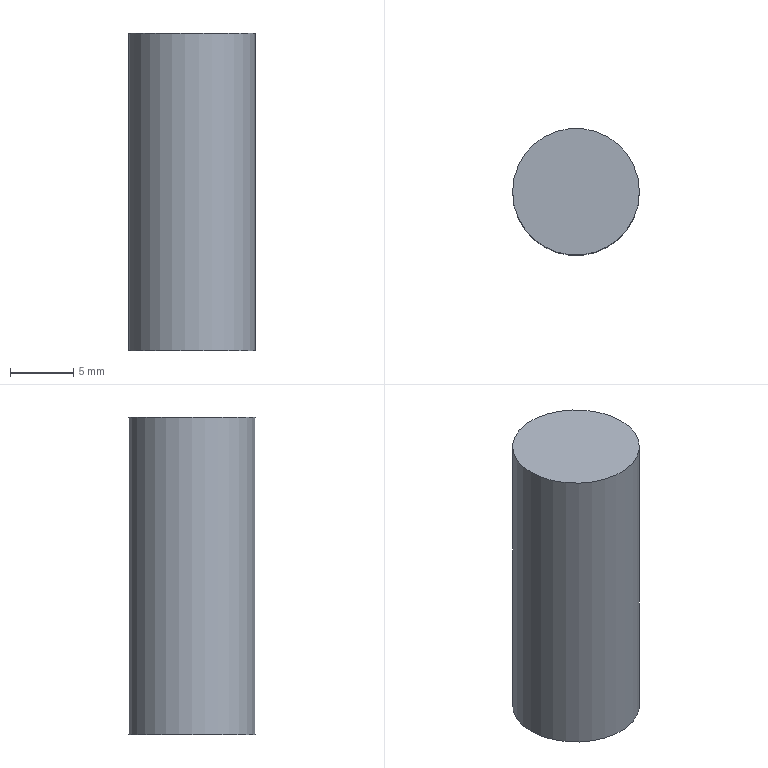Part | STEP file | xiaoding | 1 solid | 3 faces | box 10 x 10 x 25 mm | volume 1963 mm3 | plane 2 | cylinder 1 | commonest cylinder face diameters 10 x1
STEP:
#1=CARTESIAN_POINT('',(0.,0.,0.));
#2=DIRECTION('',(0.,0.,1.));
#3=DIRECTION('',(1.,0.,0.));
#4=AXIS2_PLACEMENT_3D('',#1,#2,#3);
#5=CARTESIAN_POINT('',(5.,0.,25.));
#6=VERTEX_POINT('',#5);
#7=CARTESIAN_POINT('',(0.,0.,25.));
#8=DIRECTION('',(0.,0.,1.));
#9=DIRECTION('',(1.,0.,0.));
#10=AXIS2_PLACEMENT_3D('',#7,#8,#9);
#11=CIRCLE('',#10,5.);
#12=CARTESIAN_POINT('',(0.,0.,25.));
#13=DIRECTION('',(0.,0.,-1.));
#14=DIRECTION('',(-1.,0.,0.));
#15=AXIS2_PLACEMENT_3D('',#12,#13,#14);
#16=CYLINDRICAL_SURFACE('',#15,5.);
#17=CARTESIAN_POINT('',(9.425,0.));
#18=DIRECTION('',(-1.,0.));
#19=VECTOR('',#18,1.);
#20=LINE('',#17,#19);
#21=(GEOMETRIC_REPRESENTATION_CONTEXT(2)PARAMETRIC_REPRESENTATION_CONTEXT()REPRESENTATION_CONTEXT('',''));
#22=DEFINITIONAL_REPRESENTATION('',(#20),#21);
#23=PCURVE('',#16,#22);
#24=CARTESIAN_POINT('',(0.,0.,25.));
#25=DIRECTION('',(0.,0.,1.));
#26=DIRECTION('',(1.,0.,0.));
#27=AXIS2_PLACEMENT_3D('',#24,#25,#26);
#28=PLANE('',#27);
#29=CARTESIAN_POINT('',(0.,0.));
#30=DIRECTION('',(1.,0.));
#31=AXIS2_PLACEMENT_2D('',#29,#30);
#32=CIRCLE('',#31,5.);
#33=(GEOMETRIC_REPRESENTATION_CONTEXT(2)PARAMETRIC_REPRESENTATION_CONTEXT()REPRESENTATION_CONTEXT('',''));
#34=DEFINITIONAL_REPRESENTATION('',(#32),#33);
#35=PCURVE('',#28,#34);
#36=SURFACE_CURVE('',#11,(#23,#35),.PCURVE_S1.);
#37=EDGE_CURVE('',#6,#6,#36,.T.);
#38=ORIENTED_EDGE('',*,*,#37,.F.);
#39=CARTESIAN_POINT('',(5.,0.,0.));
#40=VERTEX_POINT('',#39);
#41=CARTESIAN_POINT('',(5.,0.,25.));
#42=CARTESIAN_POINT('',(5.,0.,0.));
#43=B_SPLINE_CURVE_WITH_KNOTS('',1,(#41,#42),.UNSPECIFIED.,.F.,.F.,(2,2),(0.,25.),.PIECEWISE_BEZIER_KNOTS.);
#44=CARTESIAN_POINT('',(9.425,0.));
#45=DIRECTION('',(0.,1.));
#46=VECTOR('',#45,1.);
#47=LINE('',#44,#46);
#48=(GEOMETRIC_REPRESENTATION_CONTEXT(2)PARAMETRIC_REPRESENTATION_CONTEXT()REPRESENTATION_CONTEXT('',''));
#49=DEFINITIONAL_REPRESENTATION('',(#47),#48);
#50=PCURVE('',#16,#49);
#51=CARTESIAN_POINT('',(3.142,0.));
#52=DIRECTION('',(0.,1.));
#53=VECTOR('',#52,1.);
#54=LINE('',#51,#53);
#55=(GEOMETRIC_REPRESENTATION_CONTEXT(2)PARAMETRIC_REPRESENTATION_CONTEXT()REPRESENTATION_CONTEXT('',''));
#56=DEFINITIONAL_REPRESENTATION('',(#54),#55);
#57=PCURVE('',#16,#56);
#58=SEAM_CURVE('',#43,(#50,#57),.PCURVE_S1.);
#59=EDGE_CURVE('',#6,#40,#58,.T.);
#60=ORIENTED_EDGE('',*,*,#59,.T.);
#61=CARTESIAN_POINT('',(0.,0.,0.));
#62=DIRECTION('',(0.,0.,1.));
#63=DIRECTION('',(1.,0.,0.));
#64=AXIS2_PLACEMENT_3D('',#61,#62,#63);
#65=CIRCLE('',#64,5.);
#66=CARTESIAN_POINT('',(9.425,25.));
#67=DIRECTION('',(-1.,0.));
#68=VECTOR('',#67,1.);
#69=LINE('',#66,#68);
#70=(GEOMETRIC_REPRESENTATION_CONTEXT(2)PARAMETRIC_REPRESENTATION_CONTEXT()REPRESENTATION_CONTEXT('',''));
#71=DEFINITIONAL_REPRESENTATION('',(#69),#70);
#72=PCURVE('',#16,#71);
#73=CARTESIAN_POINT('',(0.,0.,0.));
#74=DIRECTION('',(0.,0.,1.));
#75=DIRECTION('',(1.,0.,0.));
#76=AXIS2_PLACEMENT_3D('',#73,#74,#75);
#77=PLANE('',#76);
#78=CARTESIAN_POINT('',(0.,0.));
#79=DIRECTION('',(1.,0.));
#80=AXIS2_PLACEMENT_2D('',#78,#79);
#81=CIRCLE('',#80,5.);
#82=(GEOMETRIC_REPRESENTATION_CONTEXT(2)PARAMETRIC_REPRESENTATION_CONTEXT()REPRESENTATION_CONTEXT('',''));
#83=DEFINITIONAL_REPRESENTATION('',(#81),#82);
#84=PCURVE('',#77,#83);
#85=SURFACE_CURVE('',#65,(#72,#84),.PCURVE_S1.);
#86=EDGE_CURVE('',#40,#40,#85,.T.);
#87=ORIENTED_EDGE('',*,*,#86,.T.);
#88=ORIENTED_EDGE('',*,*,#59,.F.);
#89=EDGE_LOOP('',(#38,#60,#87,#88));
#90=FACE_BOUND('',#89,.T.);
#91=ADVANCED_FACE('',(#90),#16,.T.);
#92=ORIENTED_EDGE('',*,*,#37,.T.);
#93=EDGE_LOOP('',(#92));
#94=FACE_BOUND('',#93,.T.);
#95=ADVANCED_FACE('',(#94),#28,.T.);
#96=ORIENTED_EDGE('',*,*,#86,.F.);
#97=EDGE_LOOP('',(#96));
#98=FACE_BOUND('',#97,.T.);
#99=ADVANCED_FACE('',(#98),#77,.F.);
#100=CLOSED_SHELL('',(#91,#95,#99));
#101=MANIFOLD_SOLID_BREP('',#100);
#102=(LENGTH_UNIT()NAMED_UNIT(*)SI_UNIT(.MILLI.,.METRE.));
#103=UNCERTAINTY_MEASURE_WITH_UNIT(LENGTH_MEASURE(0.00001),#102,'','');
#104=(NAMED_UNIT(*)PLANE_ANGLE_UNIT()SI_UNIT($,.RADIAN.));
#105=(NAMED_UNIT(*)SI_UNIT($,.STERADIAN.)SOLID_ANGLE_UNIT());
#106=(GEOMETRIC_REPRESENTATION_CONTEXT(3)GLOBAL_UNCERTAINTY_ASSIGNED_CONTEXT((#103))GLOBAL_UNIT_ASSIGNED_CONTEXT((#102,#104,#105))REPRESENTATION_CONTEXT('',''));
#107=ADVANCED_BREP_SHAPE_REPRESENTATION('',(#4,#101),#106);